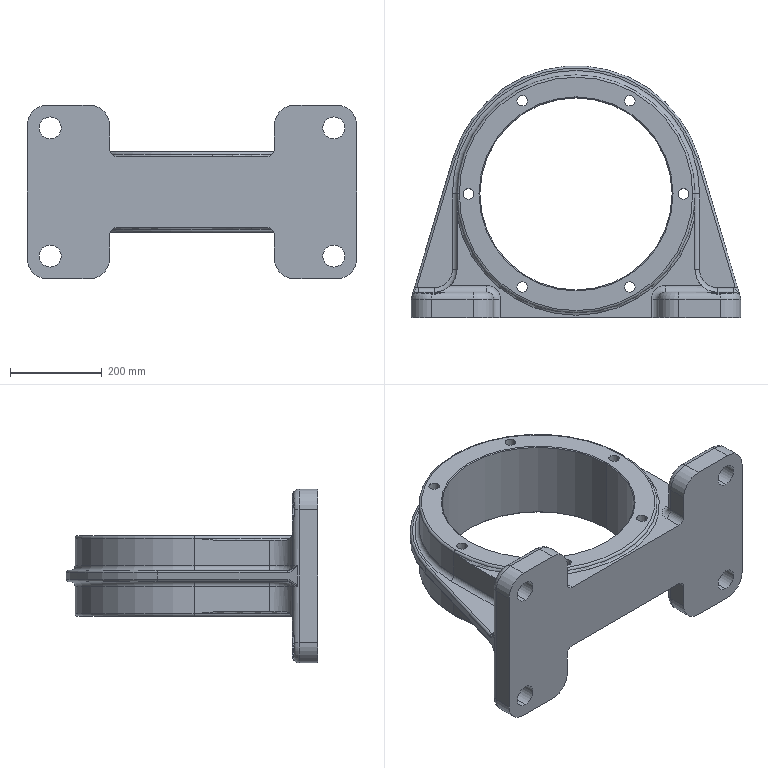Part | SolidWorks | features Fillet 10, ICE 6, Chamfer 1, CirPattern 1, Extrusion 1, LPattern 1 | 1 solid | 144 faces | box 720 x 550 x 380 mm | volume 24618968 mm3 | cylinder 75 | plane 31 | torus 30 | cone 4 | spline 4 | commonest cylinder face diameters 30 x18 90 x16 23 x12 20 x8 48 x8 10 x4